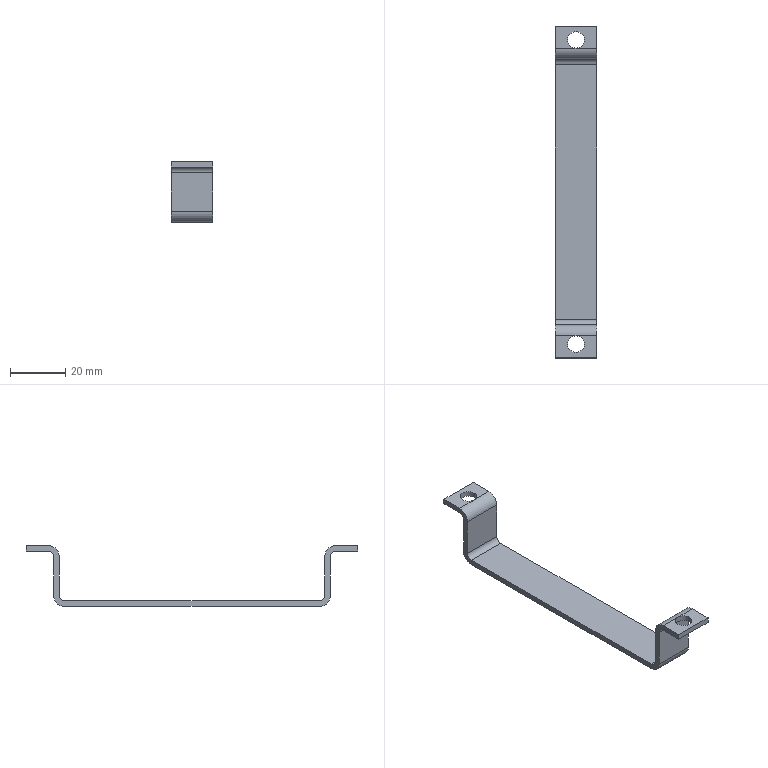Part | NX | features solid 2 | 1 solid | 26 faces | box 15 x 120 x 22 mm | volume 4532 mm3 | plane 14 | cylinder 12 | commonest cylinder face diameters 4 x4 6 x4 8 x4
STEP:
#1=CARTESIAN_POINT('',(-1005.5,255.,1293.));
#2=VERTEX_POINT('',#1);
#3=CARTESIAN_POINT('',(-1005.5,255.,1295.));
#4=VERTEX_POINT('',#3);
#5=CARTESIAN_POINT('',(-1005.5,255.,1395.919));
#6=DIRECTION('',(0.,0.,-1.));
#7=VECTOR('',#6,1000.);
#8=LINE('',#5,#7);
#9=EDGE_CURVE('',#2,#4,#8,.F.);
#10=ORIENTED_EDGE('',*,*,#9,.T.);
#11=CARTESIAN_POINT('',(-1002.5,252.,1295.));
#12=VERTEX_POINT('',#11);
#13=CARTESIAN_POINT('',(-1002.5,255.,1295.));
#14=DIRECTION('',(0.,0.,-1.));
#15=DIRECTION('',(1.,0.,0.));
#16=AXIS2_PLACEMENT_3D('',#13,#14,#15);
#17=CIRCLE('',#16,3.);
#18=EDGE_CURVE('',#12,#4,#17,.T.);
#19=ORIENTED_EDGE('',*,*,#18,.F.);
#20=CARTESIAN_POINT('',(-999.5,255.,1295.));
#21=VERTEX_POINT('',#20);
#22=CARTESIAN_POINT('',(-1002.5,255.,1295.));
#23=DIRECTION('',(0.,0.,-1.));
#24=DIRECTION('',(1.,0.,0.));
#25=AXIS2_PLACEMENT_3D('',#22,#23,#24);
#26=CIRCLE('',#25,3.);
#27=EDGE_CURVE('',#21,#12,#26,.T.);
#28=ORIENTED_EDGE('',*,*,#27,.F.);
#29=CARTESIAN_POINT('',(-999.5,255.,1293.));
#30=VERTEX_POINT('',#29);
#31=CARTESIAN_POINT('',(-999.5,255.,1395.919));
#32=DIRECTION('',(0.,0.,-1.));
#33=VECTOR('',#32,1000.);
#34=LINE('',#31,#33);
#35=EDGE_CURVE('',#21,#30,#34,.T.);
#36=ORIENTED_EDGE('',*,*,#35,.T.);
#37=CARTESIAN_POINT('',(-1002.5,252.,1293.));
#38=VERTEX_POINT('',#37);
#39=CARTESIAN_POINT('',(-1002.5,255.,1293.));
#40=DIRECTION('',(0.,0.,-1.));
#41=DIRECTION('',(1.,0.,0.));
#42=AXIS2_PLACEMENT_3D('',#39,#40,#41);
#43=CIRCLE('',#42,3.);
#44=EDGE_CURVE('',#30,#38,#43,.T.);
#45=ORIENTED_EDGE('',*,*,#44,.T.);
#46=CARTESIAN_POINT('',(-1002.5,255.,1293.));
#47=DIRECTION('',(0.,0.,-1.));
#48=DIRECTION('',(1.,0.,0.));
#49=AXIS2_PLACEMENT_3D('',#46,#47,#48);
#50=CIRCLE('',#49,3.);
#51=EDGE_CURVE('',#38,#2,#50,.T.);
#52=ORIENTED_EDGE('',*,*,#51,.T.);
#53=EDGE_LOOP('',(#10,#19,#28,#36,#45,#52));
#54=FACE_BOUND('',#53,.T.);
#55=CARTESIAN_POINT('',(-1002.5,255.,1395.919));
#56=DIRECTION('',(0.,0.,-1.));
#57=DIRECTION('',(1.,0.,0.));
#58=AXIS2_PLACEMENT_3D('',#55,#56,#57);
#59=CYLINDRICAL_SURFACE('',#58,3.);
#60=ADVANCED_FACE('',(#54),#59,.F.);
#61=CARTESIAN_POINT('',(-1005.5,145.,1295.));
#62=VERTEX_POINT('',#61);
#63=CARTESIAN_POINT('',(-1005.5,145.,1293.));
#64=VERTEX_POINT('',#63);
#65=CARTESIAN_POINT('',(-1005.5,145.,1395.919));
#66=DIRECTION('',(0.,0.,-1.));
#67=VECTOR('',#66,1000.);
#68=LINE('',#65,#67);
#69=EDGE_CURVE('',#62,#64,#68,.T.);
#70=ORIENTED_EDGE('',*,*,#69,.F.);
#71=CARTESIAN_POINT('',(-999.5,145.,1295.));
#72=VERTEX_POINT('',#71);
#73=CARTESIAN_POINT('',(-1002.5,145.,1295.));
#74=DIRECTION('',(0.,0.,-1.));
#75=DIRECTION('',(0.,1.,0.));
#76=AXIS2_PLACEMENT_3D('',#73,#74,#75);
#77=CIRCLE('',#76,3.);
#78=EDGE_CURVE('',#72,#62,#77,.T.);
#79=ORIENTED_EDGE('',*,*,#78,.F.);
#80=CARTESIAN_POINT('',(-999.5,145.,1293.));
#81=VERTEX_POINT('',#80);
#82=CARTESIAN_POINT('',(-999.5,145.,1395.919));
#83=DIRECTION('',(0.,0.,-1.));
#84=VECTOR('',#83,1000.);
#85=LINE('',#82,#84);
#86=EDGE_CURVE('',#81,#72,#85,.F.);
#87=ORIENTED_EDGE('',*,*,#86,.F.);
#88=CARTESIAN_POINT('',(-1002.5,145.,1293.));
#89=DIRECTION('',(0.,0.,-1.));
#90=DIRECTION('',(0.,1.,0.));
#91=AXIS2_PLACEMENT_3D('',#88,#89,#90);
#92=CIRCLE('',#91,3.);
#93=EDGE_CURVE('',#81,#64,#92,.T.);
#94=ORIENTED_EDGE('',*,*,#93,.T.);
#95=EDGE_LOOP('',(#70,#79,#87,#94));
#96=FACE_BOUND('',#95,.T.);
#97=CARTESIAN_POINT('',(-1002.5,145.,1395.919));
#98=DIRECTION('',(0.,0.,-1.));
#99=DIRECTION('',(1.,0.,0.));
#100=AXIS2_PLACEMENT_3D('',#97,#98,#99);
#101=CYLINDRICAL_SURFACE('',#100,3.);
#102=ADVANCED_FACE('',(#96),#101,.F.);
#103=CARTESIAN_POINT('',(-1010.,252.,1295.));
#104=VERTEX_POINT('',#103);
#105=CARTESIAN_POINT('',(-1010.,252.,1295.));
#106=DIRECTION('',(1.,0.,0.));
#107=VECTOR('',#106,1000.);
#108=LINE('',#105,#107);
#109=EDGE_CURVE('',#104,#12,#108,.T.);
#110=ORIENTED_EDGE('',*,*,#109,.T.);
#111=ORIENTED_EDGE('',*,*,#18,.T.);
#112=CARTESIAN_POINT('',(-1002.5,255.,1295.));
#113=DIRECTION('',(0.,0.,-1.));
#114=DIRECTION('',(1.,0.,0.));
#115=AXIS2_PLACEMENT_3D('',#112,#113,#114);
#116=CIRCLE('',#115,3.);
#117=EDGE_CURVE('',#4,#21,#116,.T.);
#118=ORIENTED_EDGE('',*,*,#117,.T.);
#119=ORIENTED_EDGE('',*,*,#27,.T.);
#120=CARTESIAN_POINT('',(-995.,252.,1295.));
#121=VERTEX_POINT('',#120);
#122=CARTESIAN_POINT('',(-1010.,252.,1295.));
#123=DIRECTION('',(1.,0.,0.));
#124=VECTOR('',#123,1000.);
#125=LINE('',#122,#124);
#126=EDGE_CURVE('',#12,#121,#125,.T.);
#127=ORIENTED_EDGE('',*,*,#126,.T.);
#128=CARTESIAN_POINT('',(-995.,260.,1295.));
#129=VERTEX_POINT('',#128);
#130=CARTESIAN_POINT('',(-995.,250.,1295.));
#131=DIRECTION('',(0.,1.,0.));
#132=VECTOR('',#131,1000.);
#133=LINE('',#130,#132);
#134=EDGE_CURVE('',#121,#129,#133,.T.);
#135=ORIENTED_EDGE('',*,*,#134,.T.);
#136=CARTESIAN_POINT('',(-1010.,260.,1295.));
#137=VERTEX_POINT('',#136);
#138=CARTESIAN_POINT('',(-1010.,260.,1295.));
#139=DIRECTION('',(1.,0.,0.));
#140=VECTOR('',#139,1000.);
#141=LINE('',#138,#140);
#142=EDGE_CURVE('',#137,#129,#141,.T.);
#143=ORIENTED_EDGE('',*,*,#142,.F.);
#144=CARTESIAN_POINT('',(-1010.,250.,1295.));
#145=DIRECTION('',(0.,1.,0.));
#146=VECTOR('',#145,1000.);
#147=LINE('',#144,#146);
#148=EDGE_CURVE('',#104,#137,#147,.T.);
#149=ORIENTED_EDGE('',*,*,#148,.F.);
#150=EDGE_LOOP('',(#110,#111,#118,#119,#127,#135,#143,#149));
#151=FACE_BOUND('',#150,.T.);
#152=CARTESIAN_POINT('',(-1010.,250.,1295.));
#153=DIRECTION('',(0.,0.,-1.));
#154=DIRECTION('',(-1.,0.,0.));
#155=AXIS2_PLACEMENT_3D('',#152,#153,#154);
#156=PLANE('',#155);
#157=ADVANCED_FACE('',(#151),#156,.F.);
#158=CARTESIAN_POINT('',(-995.,248.,1291.));
#159=VERTEX_POINT('',#158);
#160=CARTESIAN_POINT('',(-995.,252.,1291.));
#161=DIRECTION('',(-1.,0.,0.));
#162=DIRECTION('',(0.,0.,1.));
#163=AXIS2_PLACEMENT_3D('',#160,#161,#162);
#164=CIRCLE('',#163,4.);
#165=EDGE_CURVE('',#159,#121,#164,.T.);
#166=ORIENTED_EDGE('',*,*,#165,.T.);
#167=ORIENTED_EDGE('',*,*,#126,.F.);
#168=ORIENTED_EDGE('',*,*,#109,.F.);
#169=CARTESIAN_POINT('',(-1010.,248.,1291.));
#170=VERTEX_POINT('',#169);
#171=CARTESIAN_POINT('',(-1010.,252.,1291.));
#172=DIRECTION('',(-1.,0.,0.));
#173=DIRECTION('',(0.,0.,1.));
#174=AXIS2_PLACEMENT_3D('',#171,#172,#173);
#175=CIRCLE('',#174,4.);
#176=EDGE_CURVE('',#170,#104,#175,.T.);
#177=ORIENTED_EDGE('',*,*,#176,.F.);
#178=CARTESIAN_POINT('',(-1010.,248.,1291.));
#179=DIRECTION('',(1.,0.,0.));
#180=VECTOR('',#179,1000.);
#181=LINE('',#178,#180);
#182=EDGE_CURVE('',#170,#159,#181,.T.);
#183=ORIENTED_EDGE('',*,*,#182,.T.);
#184=EDGE_LOOP('',(#166,#167,#168,#177,#183));
#185=FACE_BOUND('',#184,.T.);
#186=CARTESIAN_POINT('',(-1010.,252.,1291.));
#187=DIRECTION('',(1.,0.,0.));
#188=DIRECTION('',(0.,0.,1.));
#189=AXIS2_PLACEMENT_3D('',#186,#187,#188);
#190=CYLINDRICAL_SURFACE('',#189,4.);
#191=ADVANCED_FACE('',(#185),#190,.T.);
#192=CARTESIAN_POINT('',(-995.,248.,1277.));
#193=VERTEX_POINT('',#192);
#194=CARTESIAN_POINT('',(-995.,248.,1273.));
#195=DIRECTION('',(0.,0.,1.));
#196=VECTOR('',#195,1000.);
#197=LINE('',#194,#196);
#198=EDGE_CURVE('',#193,#159,#197,.T.);
#199=ORIENTED_EDGE('',*,*,#198,.T.);
#200=ORIENTED_EDGE('',*,*,#182,.F.);
#201=CARTESIAN_POINT('',(-1010.,248.,1277.));
#202=VERTEX_POINT('',#201);
#203=CARTESIAN_POINT('',(-1010.,248.,1273.));
#204=DIRECTION('',(0.,0.,1.));
#205=VECTOR('',#204,1000.);
#206=LINE('',#203,#205);
#207=EDGE_CURVE('',#202,#170,#206,.T.);
#208=ORIENTED_EDGE('',*,*,#207,.F.);
#209=CARTESIAN_POINT('',(-1010.,248.,1277.));
#210=DIRECTION('',(1.,0.,0.));
#211=VECTOR('',#210,1000.);
#212=LINE('',#209,#211);
#213=EDGE_CURVE('',#202,#193,#212,.T.);
#214=ORIENTED_EDGE('',*,*,#213,.T.);
#215=EDGE_LOOP('',(#199,#200,#208,#214));
#216=FACE_BOUND('',#215,.T.);
#217=CARTESIAN_POINT('',(-1010.,248.,1273.));
#218=DIRECTION('',(0.,1.,0.));
#219=DIRECTION('',(1.,0.,0.));
#220=AXIS2_PLACEMENT_3D('',#217,#218,#219);
#221=PLANE('',#220);
#222=ADVANCED_FACE('',(#216),#221,.F.);
#223=CARTESIAN_POINT('',(-995.,246.,1275.));
#224=VERTEX_POINT('',#223);
#225=CARTESIAN_POINT('',(-995.,246.,1277.));
#226=DIRECTION('',(1.,0.,0.));
#227=DIRECTION('',(0.,0.,1.));
#228=AXIS2_PLACEMENT_3D('',#225,#226,#227);
#229=CIRCLE('',#228,2.);
#230=EDGE_CURVE('',#224,#193,#229,.T.);
#231=ORIENTED_EDGE('',*,*,#230,.T.);
#232=ORIENTED_EDGE('',*,*,#213,.F.);
#233=CARTESIAN_POINT('',(-1010.,246.,1275.));
#234=VERTEX_POINT('',#233);
#235=CARTESIAN_POINT('',(-1010.,246.,1277.));
#236=DIRECTION('',(1.,0.,0.));
#237=DIRECTION('',(0.,0.,1.));
#238=AXIS2_PLACEMENT_3D('',#235,#236,#237);
#239=CIRCLE('',#238,2.);
#240=EDGE_CURVE('',#234,#202,#239,.T.);
#241=ORIENTED_EDGE('',*,*,#240,.F.);
#242=CARTESIAN_POINT('',(-1010.,246.,1275.));
#243=DIRECTION('',(1.,0.,0.));
#244=VECTOR('',#243,1000.);
#245=LINE('',#242,#244);
#246=EDGE_CURVE('',#234,#224,#245,.T.);
#247=ORIENTED_EDGE('',*,*,#246,.T.);
#248=EDGE_LOOP('',(#231,#232,#241,#247));
#249=FACE_BOUND('',#248,.T.);
#250=CARTESIAN_POINT('',(-1010.,246.,1277.));
#251=DIRECTION('',(1.,0.,0.));
#252=DIRECTION('',(0.,0.,1.));
#253=AXIS2_PLACEMENT_3D('',#250,#251,#252);
#254=CYLINDRICAL_SURFACE('',#253,2.);
#255=ADVANCED_FACE('',(#249),#254,.F.);
#256=CARTESIAN_POINT('',(-995.,154.,1275.));
#257=VERTEX_POINT('',#256);
#258=CARTESIAN_POINT('',(-995.,150.,1275.));
#259=DIRECTION('',(0.,1.,0.));
#260=VECTOR('',#259,1000.);
#261=LINE('',#258,#260);
#262=EDGE_CURVE('',#257,#224,#261,.T.);
#263=ORIENTED_EDGE('',*,*,#262,.T.);
#264=ORIENTED_EDGE('',*,*,#246,.F.);
#265=CARTESIAN_POINT('',(-1010.,154.,1275.));
#266=VERTEX_POINT('',#265);
#267=CARTESIAN_POINT('',(-1010.,150.,1275.));
#268=DIRECTION('',(0.,1.,0.));
#269=VECTOR('',#268,1000.);
#270=LINE('',#267,#269);
#271=EDGE_CURVE('',#266,#234,#270,.T.);
#272=ORIENTED_EDGE('',*,*,#271,.F.);
#273=CARTESIAN_POINT('',(-1010.,154.,1275.));
#274=DIRECTION('',(1.,0.,0.));
#275=VECTOR('',#274,1000.);
#276=LINE('',#273,#275);
#277=EDGE_CURVE('',#266,#257,#276,.T.);
#278=ORIENTED_EDGE('',*,*,#277,.T.);
#279=EDGE_LOOP('',(#263,#264,#272,#278));
#280=FACE_BOUND('',#279,.T.);
#281=CARTESIAN_POINT('',(-1010.,150.,1275.));
#282=DIRECTION('',(0.,0.,-1.));
#283=DIRECTION('',(-1.,0.,0.));
#284=AXIS2_PLACEMENT_3D('',#281,#282,#283);
#285=PLANE('',#284);
#286=ADVANCED_FACE('',(#280),#285,.F.);
#287=CARTESIAN_POINT('',(-995.,152.,1277.));
#288=VERTEX_POINT('',#287);
#289=CARTESIAN_POINT('',(-995.,154.,1277.));
#290=DIRECTION('',(1.,0.,0.));
#291=DIRECTION('',(0.,0.,1.));
#292=AXIS2_PLACEMENT_3D('',#289,#290,#291);
#293=CIRCLE('',#292,2.);
#294=EDGE_CURVE('',#288,#257,#293,.T.);
#295=ORIENTED_EDGE('',*,*,#294,.T.);
#296=ORIENTED_EDGE('',*,*,#277,.F.);
#297=CARTESIAN_POINT('',(-1010.,152.,1277.));
#298=VERTEX_POINT('',#297);
#299=CARTESIAN_POINT('',(-1010.,154.,1277.));
#300=DIRECTION('',(1.,0.,0.));
#301=DIRECTION('',(0.,0.,1.));
#302=AXIS2_PLACEMENT_3D('',#299,#300,#301);
#303=CIRCLE('',#302,2.);
#304=EDGE_CURVE('',#298,#266,#303,.T.);
#305=ORIENTED_EDGE('',*,*,#304,.F.);
#306=CARTESIAN_POINT('',(-1010.,152.,1277.));
#307=DIRECTION('',(1.,0.,0.));
#308=VECTOR('',#307,1000.);
#309=LINE('',#306,#308);
#310=EDGE_CURVE('',#298,#288,#309,.T.);
#311=ORIENTED_EDGE('',*,*,#310,.T.);
#312=EDGE_LOOP('',(#295,#296,#305,#311));
#313=FACE_BOUND('',#312,.T.);
#314=CARTESIAN_POINT('',(-1010.,154.,1277.));
#315=DIRECTION('',(1.,0.,0.));
#316=DIRECTION('',(0.,0.,1.));
#317=AXIS2_PLACEMENT_3D('',#314,#315,#316);
#318=CYLINDRICAL_SURFACE('',#317,2.);
#319=ADVANCED_FACE('',(#313),#318,.F.);
#320=CARTESIAN_POINT('',(-995.,152.,1291.));
#321=VERTEX_POINT('',#320);
#322=CARTESIAN_POINT('',(-995.,152.,1293.));
#323=DIRECTION('',(0.,0.,-1.));
#324=VECTOR('',#323,1000.);
#325=LINE('',#322,#324);
#326=EDGE_CURVE('',#321,#288,#325,.T.);
#327=ORIENTED_EDGE('',*,*,#326,.T.);
#328=ORIENTED_EDGE('',*,*,#310,.F.);
#329=CARTESIAN_POINT('',(-1010.,152.,1291.));
#330=VERTEX_POINT('',#329);
#331=CARTESIAN_POINT('',(-1010.,152.,1293.));
#332=DIRECTION('',(0.,0.,-1.));
#333=VECTOR('',#332,1000.);
#334=LINE('',#331,#333);
#335=EDGE_CURVE('',#330,#298,#334,.T.);
#336=ORIENTED_EDGE('',*,*,#335,.F.);
#337=CARTESIAN_POINT('',(-1010.,152.,1291.));
#338=DIRECTION('',(1.,0.,0.));
#339=VECTOR('',#338,1000.);
#340=LINE('',#337,#339);
#341=EDGE_CURVE('',#330,#321,#340,.T.);
#342=ORIENTED_EDGE('',*,*,#341,.T.);
#343=EDGE_LOOP('',(#327,#328,#336,#342));
#344=FACE_BOUND('',#343,.T.);
#345=CARTESIAN_POINT('',(-1010.,152.,1293.));
#346=DIRECTION('',(0.,-1.,0.));
#347=DIRECTION('',(-1.,0.,0.));
#348=AXIS2_PLACEMENT_3D('',#345,#346,#347);
#349=PLANE('',#348);
#350=ADVANCED_FACE('',(#344),#349,.F.);
#351=CARTESIAN_POINT('',(-995.,148.,1295.));
#352=VERTEX_POINT('',#351);
#353=CARTESIAN_POINT('',(-995.,148.,1291.));
#354=DIRECTION('',(-1.,0.,0.));
#355=DIRECTION('',(0.,0.,1.));
#356=AXIS2_PLACEMENT_3D('',#353,#354,#355);
#357=CIRCLE('',#356,4.);
#358=EDGE_CURVE('',#352,#321,#357,.T.);
#359=ORIENTED_EDGE('',*,*,#358,.T.);
#360=ORIENTED_EDGE('',*,*,#341,.F.);
#361=CARTESIAN_POINT('',(-1010.,148.,1295.));
#362=VERTEX_POINT('',#361);
#363=CARTESIAN_POINT('',(-1010.,148.,1291.));
#364=DIRECTION('',(-1.,0.,0.));
#365=DIRECTION('',(0.,0.,1.));
#366=AXIS2_PLACEMENT_3D('',#363,#364,#365);
#367=CIRCLE('',#366,4.);
#368=EDGE_CURVE('',#362,#330,#367,.T.);
#369=ORIENTED_EDGE('',*,*,#368,.F.);
#370=CARTESIAN_POINT('',(-1002.5,148.,1295.));
#371=VERTEX_POINT('',#370);
#372=CARTESIAN_POINT('',(-1010.,148.,1295.));
#373=DIRECTION('',(1.,0.,0.));
#374=VECTOR('',#373,1000.);
#375=LINE('',#372,#374);
#376=EDGE_CURVE('',#362,#371,#375,.T.);
#377=ORIENTED_EDGE('',*,*,#376,.T.);
#378=CARTESIAN_POINT('',(-1010.,148.,1295.));
#379=DIRECTION('',(1.,0.,0.));
#380=VECTOR('',#379,1000.);
#381=LINE('',#378,#380);
#382=EDGE_CURVE('',#371,#352,#381,.T.);
#383=ORIENTED_EDGE('',*,*,#382,.T.);
#384=EDGE_LOOP('',(#359,#360,#369,#377,#383));
#385=FACE_BOUND('',#384,.T.);
#386=CARTESIAN_POINT('',(-1010.,148.,1291.));
#387=DIRECTION('',(1.,0.,0.));
#388=DIRECTION('',(0.,0.,1.));
#389=AXIS2_PLACEMENT_3D('',#386,#387,#388);
#390=CYLINDRICAL_SURFACE('',#389,4.);
#391=ADVANCED_FACE('',(#385),#390,.T.);
#392=ORIENTED_EDGE('',*,*,#382,.F.);
#393=CARTESIAN_POINT('',(-1002.5,145.,1295.));
#394=DIRECTION('',(0.,0.,-1.));
#395=DIRECTION('',(0.,1.,0.));
#396=AXIS2_PLACEMENT_3D('',#393,#394,#395);
#397=CIRCLE('',#396,3.);
#398=EDGE_CURVE('',#371,#72,#397,.T.);
#399=ORIENTED_EDGE('',*,*,#398,.T.);
#400=ORIENTED_EDGE('',*,*,#78,.T.);
#401=CARTESIAN_POINT('',(-1002.5,145.,1295.));
#402=DIRECTION('',(0.,0.,-1.));
#403=DIRECTION('',(0.,1.,0.));
#404=AXIS2_PLACEMENT_3D('',#401,#402,#403);
#405=CIRCLE('',#404,3.);
#406=EDGE_CURVE('',#62,#371,#405,.T.);
#407=ORIENTED_EDGE('',*,*,#406,.T.);
#408=ORIENTED_EDGE('',*,*,#376,.F.);
#409=CARTESIAN_POINT('',(-1010.,140.,1295.));
#410=VERTEX_POINT('',#409);
#411=CARTESIAN_POINT('',(-1010.,150.,1295.));
#412=DIRECTION('',(0.,1.,0.));
#413=VECTOR('',#412,1000.);
#414=LINE('',#411,#413);
#415=EDGE_CURVE('',#410,#362,#414,.T.);
#416=ORIENTED_EDGE('',*,*,#415,.F.);
#417=CARTESIAN_POINT('',(-995.,140.,1295.));
#418=VERTEX_POINT('',#417);
#419=CARTESIAN_POINT('',(-1010.,140.,1295.));
#420=DIRECTION('',(1.,0.,0.));
#421=VECTOR('',#420,1000.);
#422=LINE('',#419,#421);
#423=EDGE_CURVE('',#410,#418,#422,.T.);
#424=ORIENTED_EDGE('',*,*,#423,.T.);
#425=CARTESIAN_POINT('',(-995.,150.,1295.));
#426=DIRECTION('',(0.,1.,0.));
#427=VECTOR('',#426,1000.);
#428=LINE('',#425,#427);
#429=EDGE_CURVE('',#418,#352,#428,.T.);
#430=ORIENTED_EDGE('',*,*,#429,.T.);
#431=EDGE_LOOP('',(#392,#399,#400,#407,#408,#416,#424,#430));
#432=FACE_BOUND('',#431,.T.);
#433=CARTESIAN_POINT('',(-1010.,150.,1295.));
#434=DIRECTION('',(0.,0.,-1.));
#435=DIRECTION('',(-1.,0.,0.));
#436=AXIS2_PLACEMENT_3D('',#433,#434,#435);
#437=PLANE('',#436);
#438=ADVANCED_FACE('',(#432),#437,.F.);
#439=ORIENTED_EDGE('',*,*,#423,.F.);
#440=CARTESIAN_POINT('',(-1010.,140.,1293.));
#441=VERTEX_POINT('',#440);
#442=CARTESIAN_POINT('',(-1010.,140.,1293.));
#443=DIRECTION('',(0.,0.,-1.));
#444=VECTOR('',#443,1000.);
#445=LINE('',#442,#444);
#446=EDGE_CURVE('',#410,#441,#445,.T.);
#447=ORIENTED_EDGE('',*,*,#446,.T.);
#448=CARTESIAN_POINT('',(-995.,140.,1293.));
#449=VERTEX_POINT('',#448);
#450=CARTESIAN_POINT('',(-1010.,140.,1293.));
#451=DIRECTION('',(1.,0.,0.));
#452=VECTOR('',#451,1000.);
#453=LINE('',#450,#452);
#454=EDGE_CURVE('',#441,#449,#453,.T.);
#455=ORIENTED_EDGE('',*,*,#454,.T.);
#456=CARTESIAN_POINT('',(-995.,140.,1293.));
#457=DIRECTION('',(0.,0.,-1.));
#458=VECTOR('',#457,1000.);
#459=LINE('',#456,#458);
#460=EDGE_CURVE('',#418,#449,#459,.T.);
#461=ORIENTED_EDGE('',*,*,#460,.F.);
#462=EDGE_LOOP('',(#439,#447,#455,#461));
#463=FACE_BOUND('',#462,.T.);
#464=CARTESIAN_POINT('',(-1010.,140.,1293.));
#465=DIRECTION('',(0.,1.,0.));
#466=DIRECTION('',(1.,0.,0.));
#467=AXIS2_PLACEMENT_3D('',#464,#465,#466);
#468=PLANE('',#467);
#469=ADVANCED_FACE('',(#463),#468,.F.);
#470=CARTESIAN_POINT('',(-995.,252.,1293.));
#471=VERTEX_POINT('',#470);
#472=CARTESIAN_POINT('',(-1010.,252.,1293.));
#473=DIRECTION('',(1.,0.,0.));
#474=VECTOR('',#473,1000.);
#475=LINE('',#472,#474);
#476=EDGE_CURVE('',#38,#471,#475,.T.);
#477=ORIENTED_EDGE('',*,*,#476,.F.);
#478=ORIENTED_EDGE('',*,*,#44,.F.);
#479=CARTESIAN_POINT('',(-1002.5,255.,1293.));
#480=DIRECTION('',(0.,0.,-1.));
#481=DIRECTION('',(1.,0.,0.));
#482=AXIS2_PLACEMENT_3D('',#479,#480,#481);
#483=CIRCLE('',#482,3.);
#484=EDGE_CURVE('',#2,#30,#483,.T.);
#485=ORIENTED_EDGE('',*,*,#484,.F.);
#486=ORIENTED_EDGE('',*,*,#51,.F.);
#487=CARTESIAN_POINT('',(-1010.,252.,1293.));
#488=VERTEX_POINT('',#487);
#489=CARTESIAN_POINT('',(-1010.,252.,1293.));
#490=DIRECTION('',(1.,0.,0.));
#491=VECTOR('',#490,1000.);
#492=LINE('',#489,#491);
#493=EDGE_CURVE('',#488,#38,#492,.T.);
#494=ORIENTED_EDGE('',*,*,#493,.F.);
#495=CARTESIAN_POINT('',(-1010.,260.,1293.));
#496=VERTEX_POINT('',#495);
#497=CARTESIAN_POINT('',(-1010.,250.,1293.));
#498=DIRECTION('',(0.,1.,0.));
#499=VECTOR('',#498,1000.);
#500=LINE('',#497,#499);
#501=EDGE_CURVE('',#488,#496,#500,.T.);
#502=ORIENTED_EDGE('',*,*,#501,.T.);
#503=CARTESIAN_POINT('',(-995.,260.,1293.));
#504=VERTEX_POINT('',#503);
#505=CARTESIAN_POINT('',(-1010.,260.,1293.));
#506=DIRECTION('',(1.,0.,0.));
#507=VECTOR('',#506,1000.);
#508=LINE('',#505,#507);
#509=EDGE_CURVE('',#496,#504,#508,.T.);
#510=ORIENTED_EDGE('',*,*,#509,.T.);
#511=CARTESIAN_POINT('',(-995.,250.,1293.));
#512=DIRECTION('',(0.,1.,0.));
#513=VECTOR('',#512,1000.);
#514=LINE('',#511,#513);
#515=EDGE_CURVE('',#471,#504,#514,.T.);
#516=ORIENTED_EDGE('',*,*,#515,.F.);
#517=EDGE_LOOP('',(#477,#478,#485,#486,#494,#502,#510,#516));
#518=FACE_BOUND('',#517,.T.);
#519=CARTESIAN_POINT('',(-1010.,250.,1293.));
#520=DIRECTION('',(0.,0.,-1.));
#521=DIRECTION('',(-1.,0.,0.));
#522=AXIS2_PLACEMENT_3D('',#519,#520,#521);
#523=PLANE('',#522);
#524=ADVANCED_FACE('',(#518),#523,.T.);
#525=CARTESIAN_POINT('',(-995.,250.,1291.));
#526=VERTEX_POINT('',#525);
#527=CARTESIAN_POINT('',(-995.,252.,1291.));
#528=DIRECTION('',(-1.,0.,0.));
#529=DIRECTION('',(0.,0.,1.));
#530=AXIS2_PLACEMENT_3D('',#527,#528,#529);
#531=CIRCLE('',#530,2.);
#532=EDGE_CURVE('',#526,#471,#531,.T.);
#533=ORIENTED_EDGE('',*,*,#532,.F.);
#534=CARTESIAN_POINT('',(-1010.,250.,1291.));
#535=VERTEX_POINT('',#534);
#536=CARTESIAN_POINT('',(-1010.,250.,1291.));
#537=DIRECTION('',(1.,0.,0.));
#538=VECTOR('',#537,1000.);
#539=LINE('',#536,#538);
#540=EDGE_CURVE('',#535,#526,#539,.T.);
#541=ORIENTED_EDGE('',*,*,#540,.F.);
#542=CARTESIAN_POINT('',(-1010.,252.,1291.));
#543=DIRECTION('',(-1.,0.,0.));
#544=DIRECTION('',(0.,0.,1.));
#545=AXIS2_PLACEMENT_3D('',#542,#543,#544);
#546=CIRCLE('',#545,2.);
#547=EDGE_CURVE('',#535,#488,#546,.T.);
#548=ORIENTED_EDGE('',*,*,#547,.T.);
#549=ORIENTED_EDGE('',*,*,#493,.T.);
#550=ORIENTED_EDGE('',*,*,#476,.T.);
#551=EDGE_LOOP('',(#533,#541,#548,#549,#550));
#552=FACE_BOUND('',#551,.T.);
#553=CARTESIAN_POINT('',(-1010.,252.,1291.));
#554=DIRECTION('',(1.,0.,0.));
#555=DIRECTION('',(0.,0.,1.));
#556=AXIS2_PLACEMENT_3D('',#553,#554,#555);
#557=CYLINDRICAL_SURFACE('',#556,2.);
#558=ADVANCED_FACE('',(#552),#557,.F.);
#559=CARTESIAN_POINT('',(-995.,250.,1277.));
#560=VERTEX_POINT('',#559);
#561=CARTESIAN_POINT('',(-995.,250.,1273.));
#562=DIRECTION('',(0.,0.,1.));
#563=VECTOR('',#562,1000.);
#564=LINE('',#561,#563);
#565=EDGE_CURVE('',#560,#526,#564,.T.);
#566=ORIENTED_EDGE('',*,*,#565,.F.);
#567=CARTESIAN_POINT('',(-1010.,250.,1277.));
#568=VERTEX_POINT('',#567);
#569=CARTESIAN_POINT('',(-1010.,250.,1277.));
#570=DIRECTION('',(1.,0.,0.));
#571=VECTOR('',#570,1000.);
#572=LINE('',#569,#571);
#573=EDGE_CURVE('',#568,#560,#572,.T.);
#574=ORIENTED_EDGE('',*,*,#573,.F.);
#575=CARTESIAN_POINT('',(-1010.,250.,1273.));
#576=DIRECTION('',(0.,0.,1.));
#577=VECTOR('',#576,1000.);
#578=LINE('',#575,#577);
#579=EDGE_CURVE('',#568,#535,#578,.T.);
#580=ORIENTED_EDGE('',*,*,#579,.T.);
#581=ORIENTED_EDGE('',*,*,#540,.T.);
#582=EDGE_LOOP('',(#566,#574,#580,#581));
#583=FACE_BOUND('',#582,.T.);
#584=CARTESIAN_POINT('',(-1010.,250.,1273.));
#585=DIRECTION('',(0.,1.,0.));
#586=DIRECTION('',(1.,0.,0.));
#587=AXIS2_PLACEMENT_3D('',#584,#585,#586);
#588=PLANE('',#587);
#589=ADVANCED_FACE('',(#583),#588,.T.);
#590=CARTESIAN_POINT('',(-995.,246.,1273.));
#591=VERTEX_POINT('',#590);
#592=CARTESIAN_POINT('',(-995.,246.,1277.));
#593=DIRECTION('',(1.,0.,0.));
#594=DIRECTION('',(0.,0.,-1.));
#595=AXIS2_PLACEMENT_3D('',#592,#593,#594);
#596=CIRCLE('',#595,4.);
#597=EDGE_CURVE('',#591,#560,#596,.T.);
#598=ORIENTED_EDGE('',*,*,#597,.F.);
#599=CARTESIAN_POINT('',(-1010.,246.,1273.));
#600=VERTEX_POINT('',#599);
#601=CARTESIAN_POINT('',(-1010.,246.,1273.));
#602=DIRECTION('',(1.,0.,0.));
#603=VECTOR('',#602,1000.);
#604=LINE('',#601,#603);
#605=EDGE_CURVE('',#600,#591,#604,.T.);
#606=ORIENTED_EDGE('',*,*,#605,.F.);
#607=CARTESIAN_POINT('',(-1010.,246.,1277.));
#608=DIRECTION('',(1.,0.,0.));
#609=DIRECTION('',(0.,0.,-1.));
#610=AXIS2_PLACEMENT_3D('',#607,#608,#609);
#611=CIRCLE('',#610,4.);
#612=EDGE_CURVE('',#600,#568,#611,.T.);
#613=ORIENTED_EDGE('',*,*,#612,.T.);
#614=ORIENTED_EDGE('',*,*,#573,.T.);
#615=EDGE_LOOP('',(#598,#606,#613,#614));
#616=FACE_BOUND('',#615,.T.);
#617=CARTESIAN_POINT('',(-1010.,246.,1277.));
#618=DIRECTION('',(1.,0.,0.));
#619=DIRECTION('',(0.,0.,1.));
#620=AXIS2_PLACEMENT_3D('',#617,#618,#619);
#621=CYLINDRICAL_SURFACE('',#620,4.);
#622=ADVANCED_FACE('',(#616),#621,.T.);
#623=CARTESIAN_POINT('',(-995.,154.,1273.));
#624=VERTEX_POINT('',#623);
#625=CARTESIAN_POINT('',(-995.,150.,1273.));
#626=DIRECTION('',(0.,1.,0.));
#627=VECTOR('',#626,1000.);
#628=LINE('',#625,#627);
#629=EDGE_CURVE('',#624,#591,#628,.T.);
#630=ORIENTED_EDGE('',*,*,#629,.F.);
#631=CARTESIAN_POINT('',(-1010.,154.,1273.));
#632=VERTEX_POINT('',#631);
#633=CARTESIAN_POINT('',(-1010.,154.,1273.));
#634=DIRECTION('',(1.,0.,0.));
#635=VECTOR('',#634,1000.);
#636=LINE('',#633,#635);
#637=EDGE_CURVE('',#632,#624,#636,.T.);
#638=ORIENTED_EDGE('',*,*,#637,.F.);
#639=CARTESIAN_POINT('',(-1010.,150.,1273.));
#640=DIRECTION('',(0.,1.,0.));
#641=VECTOR('',#640,1000.);
#642=LINE('',#639,#641);
#643=EDGE_CURVE('',#632,#600,#642,.T.);
#644=ORIENTED_EDGE('',*,*,#643,.T.);
#645=ORIENTED_EDGE('',*,*,#605,.T.);
#646=EDGE_LOOP('',(#630,#638,#644,#645));
#647=FACE_BOUND('',#646,.T.);
#648=CARTESIAN_POINT('',(-1010.,150.,1273.));
#649=DIRECTION('',(0.,0.,-1.));
#650=DIRECTION('',(-1.,0.,0.));
#651=AXIS2_PLACEMENT_3D('',#648,#649,#650);
#652=PLANE('',#651);
#653=ADVANCED_FACE('',(#647),#652,.T.);
#654=CARTESIAN_POINT('',(-995.,150.,1277.));
#655=VERTEX_POINT('',#654);
#656=CARTESIAN_POINT('',(-995.,154.,1277.));
#657=DIRECTION('',(1.,0.,0.));
#658=DIRECTION('',(0.,0.,-1.));
#659=AXIS2_PLACEMENT_3D('',#656,#657,#658);
#660=CIRCLE('',#659,4.);
#661=EDGE_CURVE('',#655,#624,#660,.T.);
#662=ORIENTED_EDGE('',*,*,#661,.F.);
#663=CARTESIAN_POINT('',(-1010.,150.,1277.));
#664=VERTEX_POINT('',#663);
#665=CARTESIAN_POINT('',(-1010.,150.,1277.));
#666=DIRECTION('',(1.,0.,0.));
#667=VECTOR('',#666,1000.);
#668=LINE('',#665,#667);
#669=EDGE_CURVE('',#664,#655,#668,.T.);
#670=ORIENTED_EDGE('',*,*,#669,.F.);
#671=CARTESIAN_POINT('',(-1010.,154.,1277.));
#672=DIRECTION('',(1.,0.,0.));
#673=DIRECTION('',(0.,0.,-1.));
#674=AXIS2_PLACEMENT_3D('',#671,#672,#673);
#675=CIRCLE('',#674,4.);
#676=EDGE_CURVE('',#664,#632,#675,.T.);
#677=ORIENTED_EDGE('',*,*,#676,.T.);
#678=ORIENTED_EDGE('',*,*,#637,.T.);
#679=EDGE_LOOP('',(#662,#670,#677,#678));
#680=FACE_BOUND('',#679,.T.);
#681=CARTESIAN_POINT('',(-1010.,154.,1277.));
#682=DIRECTION('',(1.,0.,0.));
#683=DIRECTION('',(0.,0.,1.));
#684=AXIS2_PLACEMENT_3D('',#681,#682,#683);
#685=CYLINDRICAL_SURFACE('',#684,4.);
#686=ADVANCED_FACE('',(#680),#685,.T.);
#687=CARTESIAN_POINT('',(-995.,150.,1291.));
#688=VERTEX_POINT('',#687);
#689=CARTESIAN_POINT('',(-995.,150.,1293.));
#690=DIRECTION('',(0.,0.,-1.));
#691=VECTOR('',#690,1000.);
#692=LINE('',#689,#691);
#693=EDGE_CURVE('',#688,#655,#692,.T.);
#694=ORIENTED_EDGE('',*,*,#693,.F.);
#695=CARTESIAN_POINT('',(-1010.,150.,1291.));
#696=VERTEX_POINT('',#695);
#697=CARTESIAN_POINT('',(-1010.,150.,1291.));
#698=DIRECTION('',(1.,0.,0.));
#699=VECTOR('',#698,1000.);
#700=LINE('',#697,#699);
#701=EDGE_CURVE('',#696,#688,#700,.T.);
#702=ORIENTED_EDGE('',*,*,#701,.F.);
#703=CARTESIAN_POINT('',(-1010.,150.,1293.));
#704=DIRECTION('',(0.,0.,-1.));
#705=VECTOR('',#704,1000.);
#706=LINE('',#703,#705);
#707=EDGE_CURVE('',#696,#664,#706,.T.);
#708=ORIENTED_EDGE('',*,*,#707,.T.);
#709=ORIENTED_EDGE('',*,*,#669,.T.);
#710=EDGE_LOOP('',(#694,#702,#708,#709));
#711=FACE_BOUND('',#710,.T.);
#712=CARTESIAN_POINT('',(-1010.,150.,1293.));
#713=DIRECTION('',(0.,-1.,0.));
#714=DIRECTION('',(-1.,0.,0.));
#715=AXIS2_PLACEMENT_3D('',#712,#713,#714);
#716=PLANE('',#715);
#717=ADVANCED_FACE('',(#711),#716,.T.);
#718=CARTESIAN_POINT('',(-995.,148.,1293.));
#719=VERTEX_POINT('',#718);
#720=CARTESIAN_POINT('',(-995.,148.,1291.));
#721=DIRECTION('',(-1.,0.,0.));
#722=DIRECTION('',(0.,0.,1.));
#723=AXIS2_PLACEMENT_3D('',#720,#721,#722);
#724=CIRCLE('',#723,2.);
#725=EDGE_CURVE('',#719,#688,#724,.T.);
#726=ORIENTED_EDGE('',*,*,#725,.F.);
#727=CARTESIAN_POINT('',(-1002.5,148.,1293.));
#728=VERTEX_POINT('',#727);
#729=CARTESIAN_POINT('',(-1010.,148.,1293.));
#730=DIRECTION('',(1.,0.,0.));
#731=VECTOR('',#730,1000.);
#732=LINE('',#729,#731);
#733=EDGE_CURVE('',#728,#719,#732,.T.);
#734=ORIENTED_EDGE('',*,*,#733,.F.);
#735=CARTESIAN_POINT('',(-1010.,148.,1293.));
#736=VERTEX_POINT('',#735);
#737=CARTESIAN_POINT('',(-1010.,148.,1293.));
#738=DIRECTION('',(1.,0.,0.));
#739=VECTOR('',#738,1000.);
#740=LINE('',#737,#739);
#741=EDGE_CURVE('',#736,#728,#740,.T.);
#742=ORIENTED_EDGE('',*,*,#741,.F.);
#743=CARTESIAN_POINT('',(-1010.,148.,1291.));
#744=DIRECTION('',(-1.,0.,0.));
#745=DIRECTION('',(0.,0.,1.));
#746=AXIS2_PLACEMENT_3D('',#743,#744,#745);
#747=CIRCLE('',#746,2.);
#748=EDGE_CURVE('',#736,#696,#747,.T.);
#749=ORIENTED_EDGE('',*,*,#748,.T.);
#750=ORIENTED_EDGE('',*,*,#701,.T.);
#751=EDGE_LOOP('',(#726,#734,#742,#749,#750));
#752=FACE_BOUND('',#751,.T.);
#753=CARTESIAN_POINT('',(-1010.,148.,1291.));
#754=DIRECTION('',(1.,0.,0.));
#755=DIRECTION('',(0.,0.,1.));
#756=AXIS2_PLACEMENT_3D('',#753,#754,#755);
#757=CYLINDRICAL_SURFACE('',#756,2.);
#758=ADVANCED_FACE('',(#752),#757,.F.);
#759=ORIENTED_EDGE('',*,*,#741,.T.);
#760=CARTESIAN_POINT('',(-1002.5,145.,1293.));
#761=DIRECTION('',(0.,0.,-1.));
#762=DIRECTION('',(0.,1.,0.));
#763=AXIS2_PLACEMENT_3D('',#760,#761,#762);
#764=CIRCLE('',#763,3.);
#765=EDGE_CURVE('',#64,#728,#764,.T.);
#766=ORIENTED_EDGE('',*,*,#765,.F.);
#767=ORIENTED_EDGE('',*,*,#93,.F.);
#768=CARTESIAN_POINT('',(-1002.5,145.,1293.));
#769=DIRECTION('',(0.,0.,-1.));
#770=DIRECTION('',(0.,1.,0.));
#771=AXIS2_PLACEMENT_3D('',#768,#769,#770);
#772=CIRCLE('',#771,3.);
#773=EDGE_CURVE('',#728,#81,#772,.T.);
#774=ORIENTED_EDGE('',*,*,#773,.F.);
#775=ORIENTED_EDGE('',*,*,#733,.T.);
#776=CARTESIAN_POINT('',(-995.,150.,1293.));
#777=DIRECTION('',(0.,1.,0.));
#778=VECTOR('',#777,1000.);
#779=LINE('',#776,#778);
#780=EDGE_CURVE('',#449,#719,#779,.T.);
#781=ORIENTED_EDGE('',*,*,#780,.F.);
#782=ORIENTED_EDGE('',*,*,#454,.F.);
#783=CARTESIAN_POINT('',(-1010.,150.,1293.));
#784=DIRECTION('',(0.,1.,0.));
#785=VECTOR('',#784,1000.);
#786=LINE('',#783,#785);
#787=EDGE_CURVE('',#441,#736,#786,.T.);
#788=ORIENTED_EDGE('',*,*,#787,.T.);
#789=EDGE_LOOP('',(#759,#766,#767,#774,#775,#781,#782,#788));
#790=FACE_BOUND('',#789,.T.);
#791=CARTESIAN_POINT('',(-1010.,150.,1293.));
#792=DIRECTION('',(0.,0.,-1.));
#793=DIRECTION('',(-1.,0.,0.));
#794=AXIS2_PLACEMENT_3D('',#791,#792,#793);
#795=PLANE('',#794);
#796=ADVANCED_FACE('',(#790),#795,.T.);
#797=ORIENTED_EDGE('',*,*,#780,.T.);
#798=ORIENTED_EDGE('',*,*,#725,.T.);
#799=ORIENTED_EDGE('',*,*,#693,.T.);
#800=ORIENTED_EDGE('',*,*,#661,.T.);
#801=ORIENTED_EDGE('',*,*,#629,.T.);
#802=ORIENTED_EDGE('',*,*,#597,.T.);
#803=ORIENTED_EDGE('',*,*,#565,.T.);
#804=ORIENTED_EDGE('',*,*,#532,.T.);
#805=ORIENTED_EDGE('',*,*,#515,.T.);
#806=CARTESIAN_POINT('',(-995.,260.,1293.));
#807=DIRECTION('',(0.,0.,-1.));
#808=VECTOR('',#807,1000.);
#809=LINE('',#806,#808);
#810=EDGE_CURVE('',#129,#504,#809,.T.);
#811=ORIENTED_EDGE('',*,*,#810,.F.);
#812=ORIENTED_EDGE('',*,*,#134,.F.);
#813=ORIENTED_EDGE('',*,*,#165,.F.);
#814=ORIENTED_EDGE('',*,*,#198,.F.);
#815=ORIENTED_EDGE('',*,*,#230,.F.);
#816=ORIENTED_EDGE('',*,*,#262,.F.);
#817=ORIENTED_EDGE('',*,*,#294,.F.);
#818=ORIENTED_EDGE('',*,*,#326,.F.);
#819=ORIENTED_EDGE('',*,*,#358,.F.);
#820=ORIENTED_EDGE('',*,*,#429,.F.);
#821=ORIENTED_EDGE('',*,*,#460,.T.);
#822=EDGE_LOOP('',(#797,#798,#799,#800,#801,#802,#803,#804,#805,#811,#812,#813,#814,#815,#816,#817,#818,#819,#820,#821));
#823=FACE_BOUND('',#822,.T.);
#824=CARTESIAN_POINT('',(-995.,150.,1293.));
#825=DIRECTION('',(-1.,0.,0.));
#826=DIRECTION('',(0.,0.,1.));
#827=AXIS2_PLACEMENT_3D('',#824,#825,#826);
#828=PLANE('',#827);
#829=ADVANCED_FACE('',(#823),#828,.F.);
#830=CARTESIAN_POINT('',(-1010.,260.,1293.));
#831=DIRECTION('',(0.,0.,-1.));
#832=VECTOR('',#831,1000.);
#833=LINE('',#830,#832);
#834=EDGE_CURVE('',#137,#496,#833,.T.);
#835=ORIENTED_EDGE('',*,*,#834,.F.);
#836=ORIENTED_EDGE('',*,*,#142,.T.);
#837=ORIENTED_EDGE('',*,*,#810,.T.);
#838=ORIENTED_EDGE('',*,*,#509,.F.);
#839=EDGE_LOOP('',(#835,#836,#837,#838));
#840=FACE_BOUND('',#839,.T.);
#841=CARTESIAN_POINT('',(-1010.,260.,1293.));
#842=DIRECTION('',(0.,1.,0.));
#843=DIRECTION('',(1.,0.,0.));
#844=AXIS2_PLACEMENT_3D('',#841,#842,#843);
#845=PLANE('',#844);
#846=ADVANCED_FACE('',(#840),#845,.T.);
#847=ORIENTED_EDGE('',*,*,#501,.F.);
#848=ORIENTED_EDGE('',*,*,#547,.F.);
#849=ORIENTED_EDGE('',*,*,#579,.F.);
#850=ORIENTED_EDGE('',*,*,#612,.F.);
#851=ORIENTED_EDGE('',*,*,#643,.F.);
#852=ORIENTED_EDGE('',*,*,#676,.F.);
#853=ORIENTED_EDGE('',*,*,#707,.F.);
#854=ORIENTED_EDGE('',*,*,#748,.F.);
#855=ORIENTED_EDGE('',*,*,#787,.F.);
#856=ORIENTED_EDGE('',*,*,#446,.F.);
#857=ORIENTED_EDGE('',*,*,#415,.T.);
#858=ORIENTED_EDGE('',*,*,#368,.T.);
#859=ORIENTED_EDGE('',*,*,#335,.T.);
#860=ORIENTED_EDGE('',*,*,#304,.T.);
#861=ORIENTED_EDGE('',*,*,#271,.T.);
#862=ORIENTED_EDGE('',*,*,#240,.T.);
#863=ORIENTED_EDGE('',*,*,#207,.T.);
#864=ORIENTED_EDGE('',*,*,#176,.T.);
#865=ORIENTED_EDGE('',*,*,#148,.T.);
#866=ORIENTED_EDGE('',*,*,#834,.T.);
#867=EDGE_LOOP('',(#847,#848,#849,#850,#851,#852,#853,#854,#855,#856,#857,#858,#859,#860,#861,#862,#863,#864,#865,#866));
#868=FACE_BOUND('',#867,.T.);
#869=CARTESIAN_POINT('',(-1010.,250.,1293.));
#870=DIRECTION('',(-1.,0.,0.));
#871=DIRECTION('',(0.,0.,1.));
#872=AXIS2_PLACEMENT_3D('',#869,#870,#871);
#873=PLANE('',#872);
#874=ADVANCED_FACE('',(#868),#873,.T.);
#875=ORIENTED_EDGE('',*,*,#406,.F.);
#876=ORIENTED_EDGE('',*,*,#69,.T.);
#877=ORIENTED_EDGE('',*,*,#765,.T.);
#878=ORIENTED_EDGE('',*,*,#773,.T.);
#879=ORIENTED_EDGE('',*,*,#86,.T.);
#880=ORIENTED_EDGE('',*,*,#398,.F.);
#881=EDGE_LOOP('',(#875,#876,#877,#878,#879,#880));
#882=FACE_BOUND('',#881,.T.);
#883=CARTESIAN_POINT('',(-1002.5,145.,1395.919));
#884=DIRECTION('',(0.,0.,-1.));
#885=DIRECTION('',(1.,0.,0.));
#886=AXIS2_PLACEMENT_3D('',#883,#884,#885);
#887=CYLINDRICAL_SURFACE('',#886,3.);
#888=ADVANCED_FACE('',(#882),#887,.F.);
#889=ORIENTED_EDGE('',*,*,#117,.F.);
#890=ORIENTED_EDGE('',*,*,#9,.F.);
#891=ORIENTED_EDGE('',*,*,#484,.T.);
#892=ORIENTED_EDGE('',*,*,#35,.F.);
#893=EDGE_LOOP('',(#889,#890,#891,#892));
#894=FACE_BOUND('',#893,.T.);
#895=CARTESIAN_POINT('',(-1002.5,255.,1395.919));
#896=DIRECTION('',(0.,0.,-1.));
#897=DIRECTION('',(1.,0.,0.));
#898=AXIS2_PLACEMENT_3D('',#895,#896,#897);
#899=CYLINDRICAL_SURFACE('',#898,3.);
#900=ADVANCED_FACE('',(#894),#899,.F.);
#901=CLOSED_SHELL('',(#60,#102,#157,#191,#222,#255,#286,#319,#350,#391,#438,#469,#524,#558,#589,#622,#653,#686,#717,#758,#796,#829,#846,#874,#888,#900));
#902=MANIFOLD_SOLID_BREP('',#901);
#903=(LENGTH_UNIT()NAMED_UNIT(*)SI_UNIT(.MILLI.,.METRE.));
#904=UNCERTAINTY_MEASURE_WITH_UNIT(LENGTH_MEASURE(0.00001),#903,'','');
#905=(NAMED_UNIT(*)PLANE_ANGLE_UNIT()SI_UNIT($,.RADIAN.));
#906=(NAMED_UNIT(*)SI_UNIT($,.STERADIAN.)SOLID_ANGLE_UNIT());
#907=(GEOMETRIC_REPRESENTATION_CONTEXT(3)GLOBAL_UNCERTAINTY_ASSIGNED_CONTEXT((#904))GLOBAL_UNIT_ASSIGNED_CONTEXT((#903,#905,#906))REPRESENTATION_CONTEXT('',''));
#908=ADVANCED_BREP_SHAPE_REPRESENTATION('',(#902),#907);